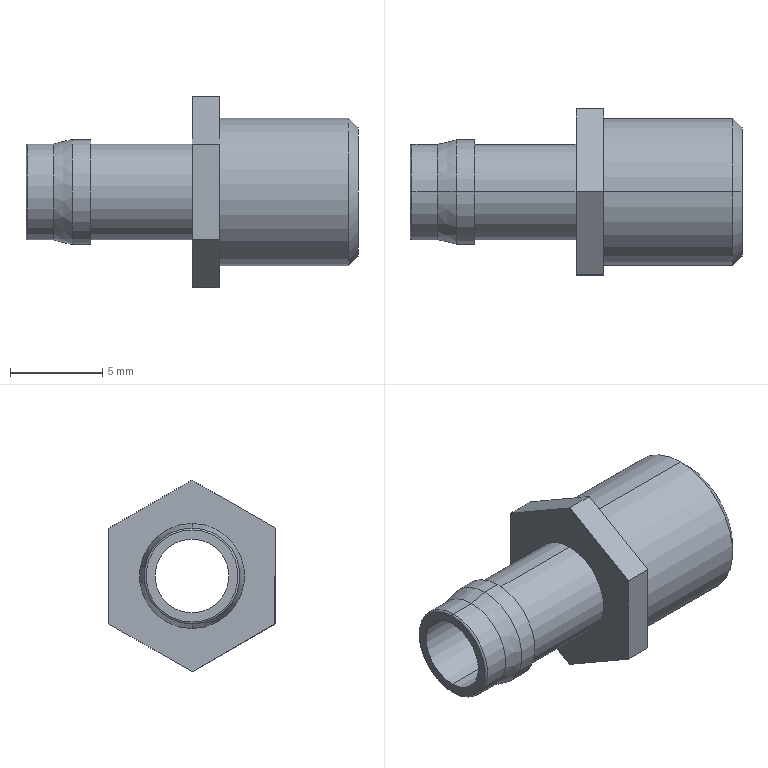Part | SolidWorks | features Chamfer 1, Fillet 1, ICE 1, Revolution 1 | 1 solid | 27 faces | box 18 x 9 x 10.392 mm | volume 450.495 mm3 | plane 11 | cylinder 10 | cone 4 | torus 2 | commonest cylinder face diameters 5.2 x4 4 x2 5.7 x2 8 x2
STEP:
#1=CARTESIAN_POINT('',(18.,0.,-3.5));
#2=VERTEX_POINT('',#1);
#3=CARTESIAN_POINT('',(18.,0.,3.5));
#4=VERTEX_POINT('',#3);
#5=CARTESIAN_POINT('',(18.,0.,0.));
#6=DIRECTION('',(1.,0.,0.));
#7=DIRECTION('',(0.,0.,1.));
#8=AXIS2_PLACEMENT_3D('',#5,#6,#7);
#9=CIRCLE('',#8,3.5);
#10=EDGE_CURVE('',#2,#4,#9,.T.);
#11=ORIENTED_EDGE('',*,*,#10,.F.);
#12=CARTESIAN_POINT('',(17.5,0.,-4.));
#13=VERTEX_POINT('',#12);
#14=CARTESIAN_POINT('',(17.5,0.,-4.));
#15=DIRECTION('',(-0.7071,0.,-0.7071));
#16=VECTOR('',#15,1000.);
#17=LINE('',#14,#16);
#18=EDGE_CURVE('',#2,#13,#17,.T.);
#19=ORIENTED_EDGE('',*,*,#18,.T.);
#20=CARTESIAN_POINT('',(17.5,0.,4.));
#21=VERTEX_POINT('',#20);
#22=CARTESIAN_POINT('',(17.5,0.,0.));
#23=DIRECTION('',(-1.,0.,0.));
#24=DIRECTION('',(0.,0.,1.));
#25=AXIS2_PLACEMENT_3D('',#22,#23,#24);
#26=CIRCLE('',#25,4.);
#27=EDGE_CURVE('',#21,#13,#26,.T.);
#28=ORIENTED_EDGE('',*,*,#27,.F.);
#29=CARTESIAN_POINT('',(17.5,0.,4.));
#30=DIRECTION('',(-0.7071,0.,0.7071));
#31=VECTOR('',#30,1000.);
#32=LINE('',#29,#31);
#33=EDGE_CURVE('',#4,#21,#32,.T.);
#34=ORIENTED_EDGE('',*,*,#33,.F.);
#35=EDGE_LOOP('',(#11,#19,#28,#34));
#36=FACE_OUTER_BOUND('',#35,.T.);
#37=CARTESIAN_POINT('',(17.5,0.,0.));
#38=DIRECTION('',(-1.,0.,0.));
#39=DIRECTION('',(0.,0.,1.));
#40=AXIS2_PLACEMENT_3D('',#37,#38,#39);
#41=CONICAL_SURFACE('',#40,4.,0.7854);
#42=ADVANCED_FACE('',(#36),#41,.T.);
#43=CARTESIAN_POINT('',(0.,0.,2.5));
#44=VERTEX_POINT('',#43);
#45=CARTESIAN_POINT('',(0.,0.,-2.5));
#46=VERTEX_POINT('',#45);
#47=CARTESIAN_POINT('',(0.,0.,0.));
#48=DIRECTION('',(-1.,0.,0.));
#49=DIRECTION('',(0.,0.,-1.));
#50=AXIS2_PLACEMENT_3D('',#47,#48,#49);
#51=CIRCLE('',#50,2.5);
#52=EDGE_CURVE('',#44,#46,#51,.T.);
#53=ORIENTED_EDGE('',*,*,#52,.F.);
#54=CARTESIAN_POINT('',(0.1,0.,2.6));
#55=VERTEX_POINT('',#54);
#56=CARTESIAN_POINT('',(0.1,0.,2.5));
#57=DIRECTION('',(0.,1.,0.));
#58=DIRECTION('',(0.,0.,1.));
#59=AXIS2_PLACEMENT_3D('',#56,#57,#58);
#60=CIRCLE('',#59,0.1);
#61=EDGE_CURVE('',#44,#55,#60,.T.);
#62=ORIENTED_EDGE('',*,*,#61,.T.);
#63=CARTESIAN_POINT('',(0.1,0.,-2.6));
#64=VERTEX_POINT('',#63);
#65=CARTESIAN_POINT('',(0.1,0.,0.));
#66=DIRECTION('',(1.,0.,0.));
#67=DIRECTION('',(0.,0.,-1.));
#68=AXIS2_PLACEMENT_3D('',#65,#66,#67);
#69=CIRCLE('',#68,2.6);
#70=EDGE_CURVE('',#64,#55,#69,.T.);
#71=ORIENTED_EDGE('',*,*,#70,.F.);
#72=CARTESIAN_POINT('',(0.1,0.,-2.5));
#73=DIRECTION('',(0.,-1.,0.));
#74=DIRECTION('',(0.,0.,-1.));
#75=AXIS2_PLACEMENT_3D('',#72,#73,#74);
#76=CIRCLE('',#75,0.1);
#77=EDGE_CURVE('',#46,#64,#76,.T.);
#78=ORIENTED_EDGE('',*,*,#77,.F.);
#79=EDGE_LOOP('',(#53,#62,#71,#78));
#80=FACE_OUTER_BOUND('',#79,.T.);
#81=CARTESIAN_POINT('',(0.1,0.,0.));
#82=DIRECTION('',(1.,0.,0.));
#83=DIRECTION('',(0.,0.,-1.));
#84=AXIS2_PLACEMENT_3D('',#81,#82,#83);
#85=TOROIDAL_SURFACE('',#84,2.5,0.1);
#86=ADVANCED_FACE('',(#80),#85,.T.);
#87=CARTESIAN_POINT('',(18.,0.,-2.));
#88=VERTEX_POINT('',#87);
#89=CARTESIAN_POINT('',(18.,0.,2.));
#90=VERTEX_POINT('',#89);
#91=CARTESIAN_POINT('',(18.,0.,0.));
#92=DIRECTION('',(-1.,0.,0.));
#93=DIRECTION('',(0.,0.,1.));
#94=AXIS2_PLACEMENT_3D('',#91,#92,#93);
#95=CIRCLE('',#94,2.);
#96=EDGE_CURVE('',#88,#90,#95,.T.);
#97=ORIENTED_EDGE('',*,*,#96,.F.);
#98=CARTESIAN_POINT('',(0.,0.,-2.));
#99=VERTEX_POINT('',#98);
#100=CARTESIAN_POINT('',(0.,0.,-2.));
#101=DIRECTION('',(-1.,0.,0.));
#102=VECTOR('',#101,1000.);
#103=LINE('',#100,#102);
#104=EDGE_CURVE('',#88,#99,#103,.T.);
#105=ORIENTED_EDGE('',*,*,#104,.T.);
#106=CARTESIAN_POINT('',(0.,0.,2.));
#107=VERTEX_POINT('',#106);
#108=CARTESIAN_POINT('',(0.,0.,0.));
#109=DIRECTION('',(-1.,0.,0.));
#110=DIRECTION('',(0.,0.,1.));
#111=AXIS2_PLACEMENT_3D('',#108,#109,#110);
#112=CIRCLE('',#111,2.);
#113=EDGE_CURVE('',#99,#107,#112,.T.);
#114=ORIENTED_EDGE('',*,*,#113,.T.);
#115=CARTESIAN_POINT('',(0.,0.,2.));
#116=DIRECTION('',(-1.,0.,0.));
#117=VECTOR('',#116,1000.);
#118=LINE('',#115,#117);
#119=EDGE_CURVE('',#90,#107,#118,.T.);
#120=ORIENTED_EDGE('',*,*,#119,.F.);
#121=EDGE_LOOP('',(#97,#105,#114,#120));
#122=FACE_OUTER_BOUND('',#121,.T.);
#123=CARTESIAN_POINT('',(0.,0.,0.));
#124=DIRECTION('',(-1.,0.,0.));
#125=DIRECTION('',(0.,0.,1.));
#126=AXIS2_PLACEMENT_3D('',#123,#124,#125);
#127=CYLINDRICAL_SURFACE('',#126,2.);
#128=ADVANCED_FACE('',(#122),#127,.F.);
#129=ORIENTED_EDGE('',*,*,#27,.T.);
#130=CARTESIAN_POINT('',(10.5,0.,-4.));
#131=VERTEX_POINT('',#130);
#132=CARTESIAN_POINT('',(0.,0.,-4.));
#133=DIRECTION('',(-1.,0.,0.));
#134=VECTOR('',#133,1000.);
#135=LINE('',#132,#134);
#136=EDGE_CURVE('',#13,#131,#135,.T.);
#137=ORIENTED_EDGE('',*,*,#136,.T.);
#138=CARTESIAN_POINT('',(10.5,0.,4.));
#139=VERTEX_POINT('',#138);
#140=CARTESIAN_POINT('',(10.5,0.,0.));
#141=DIRECTION('',(-1.,0.,0.));
#142=DIRECTION('',(0.,0.,1.));
#143=AXIS2_PLACEMENT_3D('',#140,#141,#142);
#144=CIRCLE('',#143,4.);
#145=EDGE_CURVE('',#139,#131,#144,.T.);
#146=ORIENTED_EDGE('',*,*,#145,.F.);
#147=CARTESIAN_POINT('',(0.,0.,4.));
#148=DIRECTION('',(-1.,0.,0.));
#149=VECTOR('',#148,1000.);
#150=LINE('',#147,#149);
#151=EDGE_CURVE('',#21,#139,#150,.T.);
#152=ORIENTED_EDGE('',*,*,#151,.F.);
#153=EDGE_LOOP('',(#129,#137,#146,#152));
#154=FACE_OUTER_BOUND('',#153,.T.);
#155=CARTESIAN_POINT('',(0.,0.,0.));
#156=DIRECTION('',(-1.,0.,0.));
#157=DIRECTION('',(0.,0.,1.));
#158=AXIS2_PLACEMENT_3D('',#155,#156,#157);
#159=CYLINDRICAL_SURFACE('',#158,4.);
#160=ADVANCED_FACE('',(#154),#159,.T.);
#161=CARTESIAN_POINT('',(9.,0.,2.6));
#162=VERTEX_POINT('',#161);
#163=CARTESIAN_POINT('',(9.,0.,-2.6));
#164=VERTEX_POINT('',#163);
#165=CARTESIAN_POINT('',(9.,0.,0.));
#166=DIRECTION('',(-1.,0.,0.));
#167=DIRECTION('',(0.,0.,1.));
#168=AXIS2_PLACEMENT_3D('',#165,#166,#167);
#169=CIRCLE('',#168,2.6);
#170=EDGE_CURVE('',#162,#164,#169,.T.);
#171=ORIENTED_EDGE('',*,*,#170,.T.);
#172=CARTESIAN_POINT('',(3.5,0.,-2.6));
#173=VERTEX_POINT('',#172);
#174=CARTESIAN_POINT('',(0.,0.,-2.6));
#175=DIRECTION('',(-1.,0.,0.));
#176=VECTOR('',#175,1000.);
#177=LINE('',#174,#176);
#178=EDGE_CURVE('',#164,#173,#177,.T.);
#179=ORIENTED_EDGE('',*,*,#178,.T.);
#180=CARTESIAN_POINT('',(3.5,0.,2.6));
#181=VERTEX_POINT('',#180);
#182=CARTESIAN_POINT('',(3.5,0.,0.));
#183=DIRECTION('',(-1.,0.,0.));
#184=DIRECTION('',(0.,0.,1.));
#185=AXIS2_PLACEMENT_3D('',#182,#183,#184);
#186=CIRCLE('',#185,2.6);
#187=EDGE_CURVE('',#181,#173,#186,.T.);
#188=ORIENTED_EDGE('',*,*,#187,.F.);
#189=CARTESIAN_POINT('',(0.,0.,2.6));
#190=DIRECTION('',(-1.,0.,0.));
#191=VECTOR('',#190,1000.);
#192=LINE('',#189,#191);
#193=EDGE_CURVE('',#162,#181,#192,.T.);
#194=ORIENTED_EDGE('',*,*,#193,.F.);
#195=EDGE_LOOP('',(#171,#179,#188,#194));
#196=FACE_OUTER_BOUND('',#195,.T.);
#197=CARTESIAN_POINT('',(0.,0.,0.));
#198=DIRECTION('',(-1.,0.,0.));
#199=DIRECTION('',(0.,0.,1.));
#200=AXIS2_PLACEMENT_3D('',#197,#198,#199);
#201=CYLINDRICAL_SURFACE('',#200,2.6);
#202=ADVANCED_FACE('',(#196),#201,.T.);
#203=CARTESIAN_POINT('',(3.5,0.,2.85));
#204=VERTEX_POINT('',#203);
#205=CARTESIAN_POINT('',(3.5,0.,-2.85));
#206=VERTEX_POINT('',#205);
#207=CARTESIAN_POINT('',(3.5,0.,0.));
#208=DIRECTION('',(-1.,0.,0.));
#209=DIRECTION('',(0.,0.,1.));
#210=AXIS2_PLACEMENT_3D('',#207,#208,#209);
#211=CIRCLE('',#210,2.85);
#212=EDGE_CURVE('',#204,#206,#211,.T.);
#213=ORIENTED_EDGE('',*,*,#212,.T.);
#214=CARTESIAN_POINT('',(2.5,0.,-2.85));
#215=VERTEX_POINT('',#214);
#216=CARTESIAN_POINT('',(0.,0.,-2.85));
#217=DIRECTION('',(-1.,0.,0.));
#218=VECTOR('',#217,1000.);
#219=LINE('',#216,#218);
#220=EDGE_CURVE('',#206,#215,#219,.T.);
#221=ORIENTED_EDGE('',*,*,#220,.T.);
#222=CARTESIAN_POINT('',(2.5,0.,2.85));
#223=VERTEX_POINT('',#222);
#224=CARTESIAN_POINT('',(2.5,0.,0.));
#225=DIRECTION('',(-1.,0.,0.));
#226=DIRECTION('',(0.,0.,1.));
#227=AXIS2_PLACEMENT_3D('',#224,#225,#226);
#228=CIRCLE('',#227,2.85);
#229=EDGE_CURVE('',#223,#215,#228,.T.);
#230=ORIENTED_EDGE('',*,*,#229,.F.);
#231=CARTESIAN_POINT('',(0.,0.,2.85));
#232=DIRECTION('',(-1.,0.,0.));
#233=VECTOR('',#232,1000.);
#234=LINE('',#231,#233);
#235=EDGE_CURVE('',#204,#223,#234,.T.);
#236=ORIENTED_EDGE('',*,*,#235,.F.);
#237=EDGE_LOOP('',(#213,#221,#230,#236));
#238=FACE_OUTER_BOUND('',#237,.T.);
#239=CARTESIAN_POINT('',(0.,0.,0.));
#240=DIRECTION('',(-1.,0.,0.));
#241=DIRECTION('',(0.,0.,1.));
#242=AXIS2_PLACEMENT_3D('',#239,#240,#241);
#243=CYLINDRICAL_SURFACE('',#242,2.85);
#244=ADVANCED_FACE('',(#238),#243,.T.);
#245=CARTESIAN_POINT('',(1.5,0.,2.6));
#246=VERTEX_POINT('',#245);
#247=CARTESIAN_POINT('',(1.5,0.,-2.6));
#248=VERTEX_POINT('',#247);
#249=CARTESIAN_POINT('',(1.5,0.,0.));
#250=DIRECTION('',(-1.,0.,0.));
#251=DIRECTION('',(0.,0.,1.));
#252=AXIS2_PLACEMENT_3D('',#249,#250,#251);
#253=CIRCLE('',#252,2.6);
#254=EDGE_CURVE('',#246,#248,#253,.T.);
#255=ORIENTED_EDGE('',*,*,#254,.F.);
#256=CARTESIAN_POINT('',(2.5,0.,2.85));
#257=DIRECTION('',(0.9701,0.,0.2425));
#258=VECTOR('',#257,1000.);
#259=LINE('',#256,#258);
#260=EDGE_CURVE('',#246,#223,#259,.T.);
#261=ORIENTED_EDGE('',*,*,#260,.T.);
#262=ORIENTED_EDGE('',*,*,#229,.T.);
#263=CARTESIAN_POINT('',(2.5,0.,-2.85));
#264=DIRECTION('',(0.9701,0.,-0.2425));
#265=VECTOR('',#264,1000.);
#266=LINE('',#263,#265);
#267=EDGE_CURVE('',#248,#215,#266,.T.);
#268=ORIENTED_EDGE('',*,*,#267,.F.);
#269=EDGE_LOOP('',(#255,#261,#262,#268));
#270=FACE_OUTER_BOUND('',#269,.T.);
#271=CARTESIAN_POINT('',(2.5,0.,0.));
#272=DIRECTION('',(1.,0.,0.));
#273=DIRECTION('',(0.,0.,-1.));
#274=AXIS2_PLACEMENT_3D('',#271,#272,#273);
#275=CONICAL_SURFACE('',#274,2.85,0.245);
#276=ADVANCED_FACE('',(#270),#275,.T.);
#277=ORIENTED_EDGE('',*,*,#254,.T.);
#278=CARTESIAN_POINT('',(0.,0.,-2.6));
#279=DIRECTION('',(-1.,0.,0.));
#280=VECTOR('',#279,1000.);
#281=LINE('',#278,#280);
#282=EDGE_CURVE('',#248,#64,#281,.T.);
#283=ORIENTED_EDGE('',*,*,#282,.T.);
#284=ORIENTED_EDGE('',*,*,#70,.T.);
#285=CARTESIAN_POINT('',(0.,0.,2.6));
#286=DIRECTION('',(-1.,0.,0.));
#287=VECTOR('',#286,1000.);
#288=LINE('',#285,#287);
#289=EDGE_CURVE('',#246,#55,#288,.T.);
#290=ORIENTED_EDGE('',*,*,#289,.F.);
#291=EDGE_LOOP('',(#277,#283,#284,#290));
#292=FACE_OUTER_BOUND('',#291,.T.);
#293=CARTESIAN_POINT('',(0.,0.,0.));
#294=DIRECTION('',(-1.,0.,0.));
#295=DIRECTION('',(0.,0.,1.));
#296=AXIS2_PLACEMENT_3D('',#293,#294,#295);
#297=CYLINDRICAL_SURFACE('',#296,2.6);
#298=ADVANCED_FACE('',(#292),#297,.T.);
#299=ORIENTED_EDGE('',*,*,#170,.F.);
#300=CARTESIAN_POINT('',(9.,0.,0.));
#301=DIRECTION('',(-1.,0.,0.));
#302=DIRECTION('',(0.,0.,1.));
#303=AXIS2_PLACEMENT_3D('',#300,#301,#302);
#304=CIRCLE('',#303,2.6);
#305=EDGE_CURVE('',#164,#162,#304,.T.);
#306=ORIENTED_EDGE('',*,*,#305,.F.);
#307=EDGE_LOOP('',(#299,#306));
#308=FACE_BOUND('',#307,.T.);
#309=CARTESIAN_POINT('',(9.,-4.5,2.598));
#310=VERTEX_POINT('',#309);
#311=CARTESIAN_POINT('',(9.,-4.5,-2.598));
#312=VERTEX_POINT('',#311);
#313=CARTESIAN_POINT('',(9.,-4.5,0.));
#314=DIRECTION('',(0.,0.,-1.));
#315=VECTOR('',#314,1000.);
#316=LINE('',#313,#315);
#317=EDGE_CURVE('',#310,#312,#316,.T.);
#318=ORIENTED_EDGE('',*,*,#317,.F.);
#319=CARTESIAN_POINT('',(9.,0.,5.196));
#320=VERTEX_POINT('',#319);
#321=CARTESIAN_POINT('',(9.,-0.3,5.023));
#322=DIRECTION('',(0.,-0.866,-0.5));
#323=VECTOR('',#322,1000.);
#324=LINE('',#321,#323);
#325=EDGE_CURVE('',#320,#310,#324,.T.);
#326=ORIENTED_EDGE('',*,*,#325,.F.);
#327=CARTESIAN_POINT('',(9.,4.5,2.598));
#328=VERTEX_POINT('',#327);
#329=CARTESIAN_POINT('',(9.,4.2,2.771));
#330=DIRECTION('',(0.,-0.866,0.5));
#331=VECTOR('',#330,1000.);
#332=LINE('',#329,#331);
#333=EDGE_CURVE('',#328,#320,#332,.T.);
#334=ORIENTED_EDGE('',*,*,#333,.F.);
#335=CARTESIAN_POINT('',(9.,4.5,-2.598));
#336=VERTEX_POINT('',#335);
#337=CARTESIAN_POINT('',(9.,4.5,0.));
#338=DIRECTION('',(0.,0.,1.));
#339=VECTOR('',#338,1000.);
#340=LINE('',#337,#339);
#341=EDGE_CURVE('',#336,#328,#340,.T.);
#342=ORIENTED_EDGE('',*,*,#341,.F.);
#343=CARTESIAN_POINT('',(9.,0.,-5.196));
#344=VERTEX_POINT('',#343);
#345=CARTESIAN_POINT('',(9.,4.2,-2.771));
#346=DIRECTION('',(0.,0.866,0.5));
#347=VECTOR('',#346,1000.);
#348=LINE('',#345,#347);
#349=EDGE_CURVE('',#344,#336,#348,.T.);
#350=ORIENTED_EDGE('',*,*,#349,.F.);
#351=CARTESIAN_POINT('',(9.,-0.3,-5.023));
#352=DIRECTION('',(0.,0.866,-0.5));
#353=VECTOR('',#352,1000.);
#354=LINE('',#351,#353);
#355=EDGE_CURVE('',#312,#344,#354,.T.);
#356=ORIENTED_EDGE('',*,*,#355,.F.);
#357=EDGE_LOOP('',(#318,#326,#334,#342,#350,#356));
#358=FACE_OUTER_BOUND('',#357,.T.);
#359=CARTESIAN_POINT('',(9.,2.6,0.));
#360=DIRECTION('',(1.,0.,0.));
#361=DIRECTION('',(0.,0.,-1.));
#362=AXIS2_PLACEMENT_3D('',#359,#360,#361);
#363=PLANE('',#362);
#364=ADVANCED_FACE('',(#308,#358),#363,.F.);
#365=ORIENTED_EDGE('',*,*,#145,.T.);
#366=CARTESIAN_POINT('',(10.5,0.,0.));
#367=DIRECTION('',(-1.,0.,0.));
#368=DIRECTION('',(0.,0.,1.));
#369=AXIS2_PLACEMENT_3D('',#366,#367,#368);
#370=CIRCLE('',#369,4.);
#371=EDGE_CURVE('',#131,#139,#370,.T.);
#372=ORIENTED_EDGE('',*,*,#371,.T.);
#373=EDGE_LOOP('',(#365,#372));
#374=FACE_BOUND('',#373,.T.);
#375=CARTESIAN_POINT('',(10.5,-4.5,2.598));
#376=VERTEX_POINT('',#375);
#377=CARTESIAN_POINT('',(10.5,-4.5,-2.598));
#378=VERTEX_POINT('',#377);
#379=CARTESIAN_POINT('',(10.5,-4.5,2.598));
#380=DIRECTION('',(0.,0.,-1.));
#381=VECTOR('',#380,1000.);
#382=LINE('',#379,#381);
#383=EDGE_CURVE('',#376,#378,#382,.T.);
#384=ORIENTED_EDGE('',*,*,#383,.T.);
#385=CARTESIAN_POINT('',(10.5,0.,-5.196));
#386=VERTEX_POINT('',#385);
#387=CARTESIAN_POINT('',(10.5,-4.5,-2.598));
#388=DIRECTION('',(0.,0.866,-0.5));
#389=VECTOR('',#388,1000.);
#390=LINE('',#387,#389);
#391=EDGE_CURVE('',#378,#386,#390,.T.);
#392=ORIENTED_EDGE('',*,*,#391,.T.);
#393=CARTESIAN_POINT('',(10.5,4.5,-2.598));
#394=VERTEX_POINT('',#393);
#395=CARTESIAN_POINT('',(10.5,0.,-5.196));
#396=DIRECTION('',(0.,0.866,0.5));
#397=VECTOR('',#396,1000.);
#398=LINE('',#395,#397);
#399=EDGE_CURVE('',#386,#394,#398,.T.);
#400=ORIENTED_EDGE('',*,*,#399,.T.);
#401=CARTESIAN_POINT('',(10.5,4.5,2.598));
#402=VERTEX_POINT('',#401);
#403=CARTESIAN_POINT('',(10.5,4.5,-2.598));
#404=DIRECTION('',(0.,0.,1.));
#405=VECTOR('',#404,1000.);
#406=LINE('',#403,#405);
#407=EDGE_CURVE('',#394,#402,#406,.T.);
#408=ORIENTED_EDGE('',*,*,#407,.T.);
#409=CARTESIAN_POINT('',(10.5,0.,5.196));
#410=VERTEX_POINT('',#409);
#411=CARTESIAN_POINT('',(10.5,4.5,2.598));
#412=DIRECTION('',(0.,-0.866,0.5));
#413=VECTOR('',#412,1000.);
#414=LINE('',#411,#413);
#415=EDGE_CURVE('',#402,#410,#414,.T.);
#416=ORIENTED_EDGE('',*,*,#415,.T.);
#417=CARTESIAN_POINT('',(10.5,0.,5.196));
#418=DIRECTION('',(0.,-0.866,-0.5));
#419=VECTOR('',#418,1000.);
#420=LINE('',#417,#419);
#421=EDGE_CURVE('',#410,#376,#420,.T.);
#422=ORIENTED_EDGE('',*,*,#421,.T.);
#423=EDGE_LOOP('',(#384,#392,#400,#408,#416,#422));
#424=FACE_OUTER_BOUND('',#423,.T.);
#425=CARTESIAN_POINT('',(10.5,6.,0.));
#426=DIRECTION('',(-1.,0.,0.));
#427=DIRECTION('',(0.,0.,1.));
#428=AXIS2_PLACEMENT_3D('',#425,#426,#427);
#429=PLANE('',#428);
#430=ADVANCED_FACE('',(#374,#424),#429,.F.);
#431=CARTESIAN_POINT('',(0.,0.,0.));
#432=DIRECTION('',(-1.,0.,0.));
#433=DIRECTION('',(0.,0.,-1.));
#434=AXIS2_PLACEMENT_3D('',#431,#432,#433);
#435=CIRCLE('',#434,2.5);
#436=EDGE_CURVE('',#46,#44,#435,.T.);
#437=ORIENTED_EDGE('',*,*,#436,.T.);
#438=ORIENTED_EDGE('',*,*,#52,.T.);
#439=EDGE_LOOP('',(#437,#438));
#440=FACE_OUTER_BOUND('',#439,.T.);
#441=CARTESIAN_POINT('',(0.,0.,0.));
#442=DIRECTION('',(-1.,0.,0.));
#443=DIRECTION('',(0.,0.,1.));
#444=AXIS2_PLACEMENT_3D('',#441,#442,#443);
#445=CIRCLE('',#444,2.);
#446=EDGE_CURVE('',#107,#99,#445,.T.);
#447=ORIENTED_EDGE('',*,*,#446,.F.);
#448=ORIENTED_EDGE('',*,*,#113,.F.);
#449=EDGE_LOOP('',(#447,#448));
#450=FACE_BOUND('',#449,.T.);
#451=CARTESIAN_POINT('',(0.,2.,0.));
#452=DIRECTION('',(1.,0.,0.));
#453=DIRECTION('',(0.,0.,-1.));
#454=AXIS2_PLACEMENT_3D('',#451,#452,#453);
#455=PLANE('',#454);
#456=ADVANCED_FACE('',(#440,#450),#455,.F.);
#457=ORIENTED_EDGE('',*,*,#282,.F.);
#458=CARTESIAN_POINT('',(1.5,0.,0.));
#459=DIRECTION('',(-1.,0.,0.));
#460=DIRECTION('',(0.,0.,1.));
#461=AXIS2_PLACEMENT_3D('',#458,#459,#460);
#462=CIRCLE('',#461,2.6);
#463=EDGE_CURVE('',#248,#246,#462,.T.);
#464=ORIENTED_EDGE('',*,*,#463,.T.);
#465=ORIENTED_EDGE('',*,*,#289,.T.);
#466=CARTESIAN_POINT('',(0.1,0.,0.));
#467=DIRECTION('',(1.,0.,0.));
#468=DIRECTION('',(0.,0.,-1.));
#469=AXIS2_PLACEMENT_3D('',#466,#467,#468);
#470=CIRCLE('',#469,2.6);
#471=EDGE_CURVE('',#55,#64,#470,.T.);
#472=ORIENTED_EDGE('',*,*,#471,.T.);
#473=EDGE_LOOP('',(#457,#464,#465,#472));
#474=FACE_OUTER_BOUND('',#473,.T.);
#475=CARTESIAN_POINT('',(0.,0.,0.));
#476=DIRECTION('',(-1.,0.,0.));
#477=DIRECTION('',(0.,0.,1.));
#478=AXIS2_PLACEMENT_3D('',#475,#476,#477);
#479=CYLINDRICAL_SURFACE('',#478,2.6);
#480=ADVANCED_FACE('',(#474),#479,.T.);
#481=ORIENTED_EDGE('',*,*,#260,.F.);
#482=ORIENTED_EDGE('',*,*,#463,.F.);
#483=ORIENTED_EDGE('',*,*,#267,.T.);
#484=CARTESIAN_POINT('',(2.5,0.,0.));
#485=DIRECTION('',(-1.,0.,0.));
#486=DIRECTION('',(0.,0.,1.));
#487=AXIS2_PLACEMENT_3D('',#484,#485,#486);
#488=CIRCLE('',#487,2.85);
#489=EDGE_CURVE('',#215,#223,#488,.T.);
#490=ORIENTED_EDGE('',*,*,#489,.T.);
#491=EDGE_LOOP('',(#481,#482,#483,#490));
#492=FACE_OUTER_BOUND('',#491,.T.);
#493=CARTESIAN_POINT('',(2.5,0.,0.));
#494=DIRECTION('',(1.,0.,0.));
#495=DIRECTION('',(0.,0.,-1.));
#496=AXIS2_PLACEMENT_3D('',#493,#494,#495);
#497=CONICAL_SURFACE('',#496,2.85,0.245);
#498=ADVANCED_FACE('',(#492),#497,.T.);
#499=ORIENTED_EDGE('',*,*,#220,.F.);
#500=CARTESIAN_POINT('',(3.5,0.,0.));
#501=DIRECTION('',(-1.,0.,0.));
#502=DIRECTION('',(0.,0.,1.));
#503=AXIS2_PLACEMENT_3D('',#500,#501,#502);
#504=CIRCLE('',#503,2.85);
#505=EDGE_CURVE('',#206,#204,#504,.T.);
#506=ORIENTED_EDGE('',*,*,#505,.T.);
#507=ORIENTED_EDGE('',*,*,#235,.T.);
#508=ORIENTED_EDGE('',*,*,#489,.F.);
#509=EDGE_LOOP('',(#499,#506,#507,#508));
#510=FACE_OUTER_BOUND('',#509,.T.);
#511=CARTESIAN_POINT('',(0.,0.,0.));
#512=DIRECTION('',(-1.,0.,0.));
#513=DIRECTION('',(0.,0.,1.));
#514=AXIS2_PLACEMENT_3D('',#511,#512,#513);
#515=CYLINDRICAL_SURFACE('',#514,2.85);
#516=ADVANCED_FACE('',(#510),#515,.T.);
#517=ORIENTED_EDGE('',*,*,#212,.F.);
#518=ORIENTED_EDGE('',*,*,#505,.F.);
#519=EDGE_LOOP('',(#517,#518));
#520=FACE_OUTER_BOUND('',#519,.T.);
#521=ORIENTED_EDGE('',*,*,#187,.T.);
#522=CARTESIAN_POINT('',(3.5,0.,0.));
#523=DIRECTION('',(-1.,0.,0.));
#524=DIRECTION('',(0.,0.,1.));
#525=AXIS2_PLACEMENT_3D('',#522,#523,#524);
#526=CIRCLE('',#525,2.6);
#527=EDGE_CURVE('',#173,#181,#526,.T.);
#528=ORIENTED_EDGE('',*,*,#527,.T.);
#529=EDGE_LOOP('',(#521,#528));
#530=FACE_BOUND('',#529,.T.);
#531=CARTESIAN_POINT('',(3.5,2.85,0.));
#532=DIRECTION('',(-1.,0.,0.));
#533=DIRECTION('',(0.,0.,1.));
#534=AXIS2_PLACEMENT_3D('',#531,#532,#533);
#535=PLANE('',#534);
#536=ADVANCED_FACE('',(#520,#530),#535,.F.);
#537=ORIENTED_EDGE('',*,*,#178,.F.);
#538=ORIENTED_EDGE('',*,*,#305,.T.);
#539=ORIENTED_EDGE('',*,*,#193,.T.);
#540=ORIENTED_EDGE('',*,*,#527,.F.);
#541=EDGE_LOOP('',(#537,#538,#539,#540));
#542=FACE_OUTER_BOUND('',#541,.T.);
#543=CARTESIAN_POINT('',(0.,0.,0.));
#544=DIRECTION('',(-1.,0.,0.));
#545=DIRECTION('',(0.,0.,1.));
#546=AXIS2_PLACEMENT_3D('',#543,#544,#545);
#547=CYLINDRICAL_SURFACE('',#546,2.6);
#548=ADVANCED_FACE('',(#542),#547,.T.);
#549=ORIENTED_EDGE('',*,*,#136,.F.);
#550=CARTESIAN_POINT('',(17.5,0.,0.));
#551=DIRECTION('',(-1.,0.,0.));
#552=DIRECTION('',(0.,0.,1.));
#553=AXIS2_PLACEMENT_3D('',#550,#551,#552);
#554=CIRCLE('',#553,4.);
#555=EDGE_CURVE('',#13,#21,#554,.T.);
#556=ORIENTED_EDGE('',*,*,#555,.T.);
#557=ORIENTED_EDGE('',*,*,#151,.T.);
#558=ORIENTED_EDGE('',*,*,#371,.F.);
#559=EDGE_LOOP('',(#549,#556,#557,#558));
#560=FACE_OUTER_BOUND('',#559,.T.);
#561=CARTESIAN_POINT('',(0.,0.,0.));
#562=DIRECTION('',(-1.,0.,0.));
#563=DIRECTION('',(0.,0.,1.));
#564=AXIS2_PLACEMENT_3D('',#561,#562,#563);
#565=CYLINDRICAL_SURFACE('',#564,4.);
#566=ADVANCED_FACE('',(#560),#565,.T.);
#567=CARTESIAN_POINT('',(18.,0.,0.));
#568=DIRECTION('',(1.,0.,0.));
#569=DIRECTION('',(0.,0.,1.));
#570=AXIS2_PLACEMENT_3D('',#567,#568,#569);
#571=CIRCLE('',#570,3.5);
#572=EDGE_CURVE('',#4,#2,#571,.T.);
#573=ORIENTED_EDGE('',*,*,#572,.T.);
#574=ORIENTED_EDGE('',*,*,#10,.T.);
#575=EDGE_LOOP('',(#573,#574));
#576=FACE_OUTER_BOUND('',#575,.T.);
#577=CARTESIAN_POINT('',(18.,0.,0.));
#578=DIRECTION('',(-1.,0.,0.));
#579=DIRECTION('',(0.,0.,1.));
#580=AXIS2_PLACEMENT_3D('',#577,#578,#579);
#581=CIRCLE('',#580,2.);
#582=EDGE_CURVE('',#90,#88,#581,.T.);
#583=ORIENTED_EDGE('',*,*,#582,.T.);
#584=ORIENTED_EDGE('',*,*,#96,.T.);
#585=EDGE_LOOP('',(#583,#584));
#586=FACE_BOUND('',#585,.T.);
#587=CARTESIAN_POINT('',(18.,4.,0.));
#588=DIRECTION('',(-1.,0.,0.));
#589=DIRECTION('',(0.,0.,1.));
#590=AXIS2_PLACEMENT_3D('',#587,#588,#589);
#591=PLANE('',#590);
#592=ADVANCED_FACE('',(#576,#586),#591,.F.);
#593=ORIENTED_EDGE('',*,*,#104,.F.);
#594=ORIENTED_EDGE('',*,*,#582,.F.);
#595=ORIENTED_EDGE('',*,*,#119,.T.);
#596=ORIENTED_EDGE('',*,*,#446,.T.);
#597=EDGE_LOOP('',(#593,#594,#595,#596));
#598=FACE_OUTER_BOUND('',#597,.T.);
#599=CARTESIAN_POINT('',(0.,0.,0.));
#600=DIRECTION('',(-1.,0.,0.));
#601=DIRECTION('',(0.,0.,1.));
#602=AXIS2_PLACEMENT_3D('',#599,#600,#601);
#603=CYLINDRICAL_SURFACE('',#602,2.);
#604=ADVANCED_FACE('',(#598),#603,.F.);
#605=ORIENTED_EDGE('',*,*,#317,.T.);
#606=CARTESIAN_POINT('',(0.5,-4.5,-2.598));
#607=DIRECTION('',(1.,0.,0.));
#608=VECTOR('',#607,1000.);
#609=LINE('',#606,#608);
#610=EDGE_CURVE('',#312,#378,#609,.T.);
#611=ORIENTED_EDGE('',*,*,#610,.T.);
#612=ORIENTED_EDGE('',*,*,#383,.F.);
#613=CARTESIAN_POINT('',(0.5,-4.5,2.598));
#614=DIRECTION('',(1.,0.,0.));
#615=VECTOR('',#614,1000.);
#616=LINE('',#613,#615);
#617=EDGE_CURVE('',#310,#376,#616,.T.);
#618=ORIENTED_EDGE('',*,*,#617,.F.);
#619=EDGE_LOOP('',(#605,#611,#612,#618));
#620=FACE_OUTER_BOUND('',#619,.T.);
#621=CARTESIAN_POINT('',(0.5,-4.5,2.598));
#622=DIRECTION('',(0.,-1.,0.));
#623=DIRECTION('',(0.,0.,-1.));
#624=AXIS2_PLACEMENT_3D('',#621,#622,#623);
#625=PLANE('',#624);
#626=ADVANCED_FACE('',(#620),#625,.T.);
#627=ORIENTED_EDGE('',*,*,#325,.T.);
#628=ORIENTED_EDGE('',*,*,#617,.T.);
#629=ORIENTED_EDGE('',*,*,#421,.F.);
#630=CARTESIAN_POINT('',(0.5,0.,5.196));
#631=DIRECTION('',(1.,0.,0.));
#632=VECTOR('',#631,1000.);
#633=LINE('',#630,#632);
#634=EDGE_CURVE('',#320,#410,#633,.T.);
#635=ORIENTED_EDGE('',*,*,#634,.F.);
#636=EDGE_LOOP('',(#627,#628,#629,#635));
#637=FACE_OUTER_BOUND('',#636,.T.);
#638=CARTESIAN_POINT('',(0.5,0.,5.196));
#639=DIRECTION('',(0.,-0.5,0.866));
#640=DIRECTION('',(0.,-0.866,-0.5));
#641=AXIS2_PLACEMENT_3D('',#638,#639,#640);
#642=PLANE('',#641);
#643=ADVANCED_FACE('',(#637),#642,.T.);
#644=ORIENTED_EDGE('',*,*,#333,.T.);
#645=ORIENTED_EDGE('',*,*,#634,.T.);
#646=ORIENTED_EDGE('',*,*,#415,.F.);
#647=CARTESIAN_POINT('',(0.5,4.5,2.598));
#648=DIRECTION('',(1.,0.,0.));
#649=VECTOR('',#648,1000.);
#650=LINE('',#647,#649);
#651=EDGE_CURVE('',#328,#402,#650,.T.);
#652=ORIENTED_EDGE('',*,*,#651,.F.);
#653=EDGE_LOOP('',(#644,#645,#646,#652));
#654=FACE_OUTER_BOUND('',#653,.T.);
#655=CARTESIAN_POINT('',(0.5,4.5,2.598));
#656=DIRECTION('',(0.,0.5,0.866));
#657=DIRECTION('',(0.,-0.866,0.5));
#658=AXIS2_PLACEMENT_3D('',#655,#656,#657);
#659=PLANE('',#658);
#660=ADVANCED_FACE('',(#654),#659,.T.);
#661=ORIENTED_EDGE('',*,*,#341,.T.);
#662=ORIENTED_EDGE('',*,*,#651,.T.);
#663=ORIENTED_EDGE('',*,*,#407,.F.);
#664=CARTESIAN_POINT('',(0.5,4.5,-2.598));
#665=DIRECTION('',(1.,0.,0.));
#666=VECTOR('',#665,1000.);
#667=LINE('',#664,#666);
#668=EDGE_CURVE('',#336,#394,#667,.T.);
#669=ORIENTED_EDGE('',*,*,#668,.F.);
#670=EDGE_LOOP('',(#661,#662,#663,#669));
#671=FACE_OUTER_BOUND('',#670,.T.);
#672=CARTESIAN_POINT('',(0.5,4.5,-2.598));
#673=DIRECTION('',(0.,1.,0.));
#674=DIRECTION('',(0.,0.,1.));
#675=AXIS2_PLACEMENT_3D('',#672,#673,#674);
#676=PLANE('',#675);
#677=ADVANCED_FACE('',(#671),#676,.T.);
#678=ORIENTED_EDGE('',*,*,#349,.T.);
#679=ORIENTED_EDGE('',*,*,#668,.T.);
#680=ORIENTED_EDGE('',*,*,#399,.F.);
#681=CARTESIAN_POINT('',(0.5,0.,-5.196));
#682=DIRECTION('',(1.,0.,0.));
#683=VECTOR('',#682,1000.);
#684=LINE('',#681,#683);
#685=EDGE_CURVE('',#344,#386,#684,.T.);
#686=ORIENTED_EDGE('',*,*,#685,.F.);
#687=EDGE_LOOP('',(#678,#679,#680,#686));
#688=FACE_OUTER_BOUND('',#687,.T.);
#689=CARTESIAN_POINT('',(0.5,0.,-5.196));
#690=DIRECTION('',(0.,0.5,-0.866));
#691=DIRECTION('',(0.,0.866,0.5));
#692=AXIS2_PLACEMENT_3D('',#689,#690,#691);
#693=PLANE('',#692);
#694=ADVANCED_FACE('',(#688),#693,.T.);
#695=ORIENTED_EDGE('',*,*,#355,.T.);
#696=ORIENTED_EDGE('',*,*,#685,.T.);
#697=ORIENTED_EDGE('',*,*,#391,.F.);
#698=ORIENTED_EDGE('',*,*,#610,.F.);
#699=EDGE_LOOP('',(#695,#696,#697,#698));
#700=FACE_OUTER_BOUND('',#699,.T.);
#701=CARTESIAN_POINT('',(0.5,-4.5,-2.598));
#702=DIRECTION('',(0.,-0.5,-0.866));
#703=DIRECTION('',(0.,0.866,-0.5));
#704=AXIS2_PLACEMENT_3D('',#701,#702,#703);
#705=PLANE('',#704);
#706=ADVANCED_FACE('',(#700),#705,.T.);
#707=ORIENTED_EDGE('',*,*,#61,.F.);
#708=ORIENTED_EDGE('',*,*,#436,.F.);
#709=ORIENTED_EDGE('',*,*,#77,.T.);
#710=ORIENTED_EDGE('',*,*,#471,.F.);
#711=EDGE_LOOP('',(#707,#708,#709,#710));
#712=FACE_OUTER_BOUND('',#711,.T.);
#713=CARTESIAN_POINT('',(0.1,0.,0.));
#714=DIRECTION('',(1.,0.,0.));
#715=DIRECTION('',(0.,0.,-1.));
#716=AXIS2_PLACEMENT_3D('',#713,#714,#715);
#717=TOROIDAL_SURFACE('',#716,2.5,0.1);
#718=ADVANCED_FACE('',(#712),#717,.T.);
#719=ORIENTED_EDGE('',*,*,#18,.F.);
#720=ORIENTED_EDGE('',*,*,#572,.F.);
#721=ORIENTED_EDGE('',*,*,#33,.T.);
#722=ORIENTED_EDGE('',*,*,#555,.F.);
#723=EDGE_LOOP('',(#719,#720,#721,#722));
#724=FACE_OUTER_BOUND('',#723,.T.);
#725=CARTESIAN_POINT('',(17.5,0.,0.));
#726=DIRECTION('',(-1.,0.,0.));
#727=DIRECTION('',(0.,0.,1.));
#728=AXIS2_PLACEMENT_3D('',#725,#726,#727);
#729=CONICAL_SURFACE('',#728,4.,0.7854);
#730=ADVANCED_FACE('',(#724),#729,.T.);
#731=CLOSED_SHELL('',(#42,#86,#128,#160,#202,#244,#276,#298,#364,#430,#456,#480,#498,#516,#536,#548,#566,#592,#604,#626,#643,#660,#677,#694,#706,#718,#730));
#732=MANIFOLD_SOLID_BREP('',#731);
#733=CARTESIAN_POINT('',(0.,0.,0.));
#734=DIRECTION('',(0.,0.,1.));
#735=DIRECTION('',(1.,0.,0.));
#736=AXIS2_PLACEMENT_3D('',#733,#734,#735);
#737=(LENGTH_UNIT()NAMED_UNIT(*)SI_UNIT(.MILLI.,.METRE.));
#738=UNCERTAINTY_MEASURE_WITH_UNIT(LENGTH_MEASURE(0.00001),#737,'','');
#739=(NAMED_UNIT(*)PLANE_ANGLE_UNIT()SI_UNIT($,.RADIAN.));
#740=(NAMED_UNIT(*)SI_UNIT($,.STERADIAN.)SOLID_ANGLE_UNIT());
#741=(GEOMETRIC_REPRESENTATION_CONTEXT(3)GLOBAL_UNCERTAINTY_ASSIGNED_CONTEXT((#738))GLOBAL_UNIT_ASSIGNED_CONTEXT((#737,#739,#740))REPRESENTATION_CONTEXT('',''));
#742=ADVANCED_BREP_SHAPE_REPRESENTATION('',(#732,#736),#741);